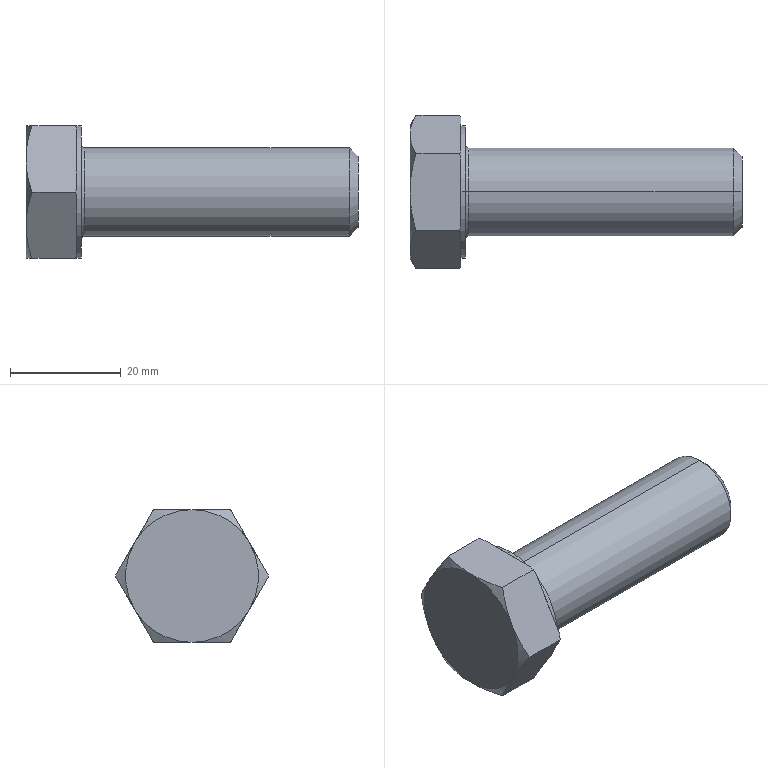Part | STEP file | Hex Head Bolt GB/T5783-2000 Fully Threaded M16x50 | 1 solid | 35 faces | box 60 x 27.713 x 24 mm | volume 14933 mm3 | plane 15 | cone 14 | cylinder 4 | torus 2 | commonest cylinder face diameters 16 x2 24 x2